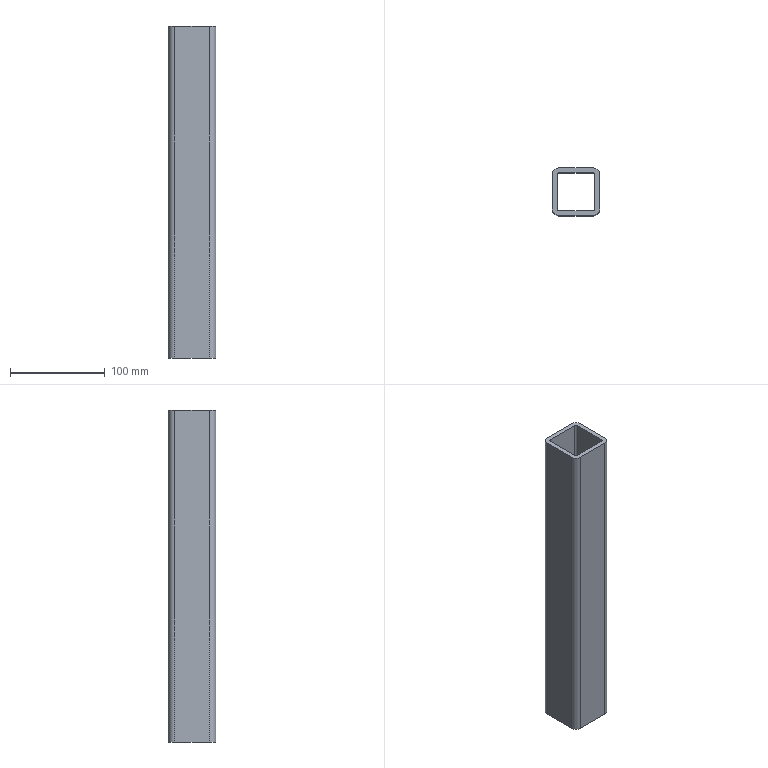Part | NX | 1 solid | 18 faces | box 50 x 50 x 350 mm | volume 301480 mm3 | plane 10 | cylinder 8 | commonest cylinder face diameters 4 x4 14 x4
STEP:
#1=CARTESIAN_POINT('',(-645.,143.,175.));
#2=VERTEX_POINT('',#1);
#3=CARTESIAN_POINT('',(-645.,143.,-175.));
#4=VERTEX_POINT('',#3);
#5=CARTESIAN_POINT('',(-645.,143.,200.));
#6=DIRECTION('',(0.,0.,-1.));
#7=VECTOR('',#6,1000.);
#8=LINE('',#5,#7);
#9=EDGE_CURVE('',#2,#4,#8,.T.);
#10=ORIENTED_EDGE('',*,*,#9,.T.);
#11=CARTESIAN_POINT('',(-645.,179.,-175.));
#12=VERTEX_POINT('',#11);
#13=CARTESIAN_POINT('',(-645.,143.,-175.));
#14=DIRECTION('',(0.,1.,0.));
#15=VECTOR('',#14,1000.);
#16=LINE('',#13,#15);
#17=EDGE_CURVE('',#4,#12,#16,.T.);
#18=ORIENTED_EDGE('',*,*,#17,.T.);
#19=CARTESIAN_POINT('',(-645.,179.,175.));
#20=VERTEX_POINT('',#19);
#21=CARTESIAN_POINT('',(-645.,179.,200.));
#22=DIRECTION('',(0.,0.,-1.));
#23=VECTOR('',#22,1000.);
#24=LINE('',#21,#23);
#25=EDGE_CURVE('',#20,#12,#24,.T.);
#26=ORIENTED_EDGE('',*,*,#25,.F.);
#27=CARTESIAN_POINT('',(-645.,143.,175.));
#28=DIRECTION('',(0.,-1.,0.));
#29=VECTOR('',#28,1000.);
#30=LINE('',#27,#29);
#31=EDGE_CURVE('',#20,#2,#30,.T.);
#32=ORIENTED_EDGE('',*,*,#31,.T.);
#33=EDGE_LOOP('',(#10,#18,#26,#32));
#34=FACE_BOUND('',#33,.T.);
#35=CARTESIAN_POINT('',(-645.,143.,200.));
#36=DIRECTION('',(1.,0.,0.));
#37=DIRECTION('',(0.,0.,-1.));
#38=AXIS2_PLACEMENT_3D('',#35,#36,#37);
#39=PLANE('',#38);
#40=ADVANCED_FACE('',(#34),#39,.T.);
#41=CARTESIAN_POINT('',(-643.,141.,175.));
#42=VERTEX_POINT('',#41);
#43=CARTESIAN_POINT('',(-643.,141.,-175.));
#44=VERTEX_POINT('',#43);
#45=CARTESIAN_POINT('',(-643.,141.,200.));
#46=DIRECTION('',(0.,0.,-1.));
#47=VECTOR('',#46,1000.);
#48=LINE('',#45,#47);
#49=EDGE_CURVE('',#42,#44,#48,.T.);
#50=ORIENTED_EDGE('',*,*,#49,.T.);
#51=CARTESIAN_POINT('',(-643.,143.,-175.));
#52=DIRECTION('',(0.,0.,-1.));
#53=DIRECTION('',(-1.,0.,0.));
#54=AXIS2_PLACEMENT_3D('',#51,#52,#53);
#55=CIRCLE('',#54,2.);
#56=EDGE_CURVE('',#44,#4,#55,.T.);
#57=ORIENTED_EDGE('',*,*,#56,.T.);
#58=ORIENTED_EDGE('',*,*,#9,.F.);
#59=CARTESIAN_POINT('',(-643.,143.,175.));
#60=DIRECTION('',(0.,0.,1.));
#61=DIRECTION('',(1.,0.,0.));
#62=AXIS2_PLACEMENT_3D('',#59,#60,#61);
#63=CIRCLE('',#62,2.);
#64=EDGE_CURVE('',#2,#42,#63,.T.);
#65=ORIENTED_EDGE('',*,*,#64,.T.);
#66=EDGE_LOOP('',(#50,#57,#58,#65));
#67=FACE_BOUND('',#66,.T.);
#68=CARTESIAN_POINT('',(-643.,143.,200.));
#69=DIRECTION('',(0.,0.,-1.));
#70=DIRECTION('',(-1.,0.,0.));
#71=AXIS2_PLACEMENT_3D('',#68,#69,#70);
#72=CYLINDRICAL_SURFACE('',#71,2.);
#73=ADVANCED_FACE('',(#67),#72,.F.);
#74=CARTESIAN_POINT('',(-607.,141.,175.));
#75=VERTEX_POINT('',#74);
#76=CARTESIAN_POINT('',(-607.,141.,-175.));
#77=VERTEX_POINT('',#76);
#78=CARTESIAN_POINT('',(-607.,141.,200.));
#79=DIRECTION('',(0.,0.,-1.));
#80=VECTOR('',#79,1000.);
#81=LINE('',#78,#80);
#82=EDGE_CURVE('',#75,#77,#81,.T.);
#83=ORIENTED_EDGE('',*,*,#82,.T.);
#84=CARTESIAN_POINT('',(-643.,141.,-175.));
#85=DIRECTION('',(-1.,0.,0.));
#86=VECTOR('',#85,1000.);
#87=LINE('',#84,#86);
#88=EDGE_CURVE('',#77,#44,#87,.T.);
#89=ORIENTED_EDGE('',*,*,#88,.T.);
#90=ORIENTED_EDGE('',*,*,#49,.F.);
#91=CARTESIAN_POINT('',(-643.,141.,175.));
#92=DIRECTION('',(1.,0.,0.));
#93=VECTOR('',#92,1000.);
#94=LINE('',#91,#93);
#95=EDGE_CURVE('',#42,#75,#94,.T.);
#96=ORIENTED_EDGE('',*,*,#95,.T.);
#97=EDGE_LOOP('',(#83,#89,#90,#96));
#98=FACE_BOUND('',#97,.T.);
#99=CARTESIAN_POINT('',(-643.,141.,200.));
#100=DIRECTION('',(0.,1.,0.));
#101=DIRECTION('',(-1.,0.,0.));
#102=AXIS2_PLACEMENT_3D('',#99,#100,#101);
#103=PLANE('',#102);
#104=ADVANCED_FACE('',(#98),#103,.T.);
#105=CARTESIAN_POINT('',(-605.,143.,175.));
#106=VERTEX_POINT('',#105);
#107=CARTESIAN_POINT('',(-605.,143.,-175.));
#108=VERTEX_POINT('',#107);
#109=CARTESIAN_POINT('',(-605.,143.,200.));
#110=DIRECTION('',(0.,0.,-1.));
#111=VECTOR('',#110,1000.);
#112=LINE('',#109,#111);
#113=EDGE_CURVE('',#106,#108,#112,.T.);
#114=ORIENTED_EDGE('',*,*,#113,.T.);
#115=CARTESIAN_POINT('',(-607.,143.,-175.));
#116=DIRECTION('',(0.,0.,-1.));
#117=DIRECTION('',(-1.,0.,0.));
#118=AXIS2_PLACEMENT_3D('',#115,#116,#117);
#119=CIRCLE('',#118,2.);
#120=EDGE_CURVE('',#108,#77,#119,.T.);
#121=ORIENTED_EDGE('',*,*,#120,.T.);
#122=ORIENTED_EDGE('',*,*,#82,.F.);
#123=CARTESIAN_POINT('',(-607.,143.,175.));
#124=DIRECTION('',(0.,0.,1.));
#125=DIRECTION('',(1.,0.,0.));
#126=AXIS2_PLACEMENT_3D('',#123,#124,#125);
#127=CIRCLE('',#126,2.);
#128=EDGE_CURVE('',#75,#106,#127,.T.);
#129=ORIENTED_EDGE('',*,*,#128,.T.);
#130=EDGE_LOOP('',(#114,#121,#122,#129));
#131=FACE_BOUND('',#130,.T.);
#132=CARTESIAN_POINT('',(-607.,143.,200.));
#133=DIRECTION('',(0.,0.,-1.));
#134=DIRECTION('',(-1.,0.,0.));
#135=AXIS2_PLACEMENT_3D('',#132,#133,#134);
#136=CYLINDRICAL_SURFACE('',#135,2.);
#137=ADVANCED_FACE('',(#131),#136,.F.);
#138=CARTESIAN_POINT('',(-605.,179.,175.));
#139=VERTEX_POINT('',#138);
#140=CARTESIAN_POINT('',(-605.,179.,-175.));
#141=VERTEX_POINT('',#140);
#142=CARTESIAN_POINT('',(-605.,179.,200.));
#143=DIRECTION('',(0.,0.,-1.));
#144=VECTOR('',#143,1000.);
#145=LINE('',#142,#144);
#146=EDGE_CURVE('',#139,#141,#145,.T.);
#147=ORIENTED_EDGE('',*,*,#146,.T.);
#148=CARTESIAN_POINT('',(-605.,179.,-175.));
#149=DIRECTION('',(0.,-1.,0.));
#150=VECTOR('',#149,1000.);
#151=LINE('',#148,#150);
#152=EDGE_CURVE('',#141,#108,#151,.T.);
#153=ORIENTED_EDGE('',*,*,#152,.T.);
#154=ORIENTED_EDGE('',*,*,#113,.F.);
#155=CARTESIAN_POINT('',(-605.,179.,175.));
#156=DIRECTION('',(0.,1.,0.));
#157=VECTOR('',#156,1000.);
#158=LINE('',#155,#157);
#159=EDGE_CURVE('',#106,#139,#158,.T.);
#160=ORIENTED_EDGE('',*,*,#159,.T.);
#161=EDGE_LOOP('',(#147,#153,#154,#160));
#162=FACE_BOUND('',#161,.T.);
#163=CARTESIAN_POINT('',(-605.,179.,200.));
#164=DIRECTION('',(-1.,0.,0.));
#165=DIRECTION('',(0.,0.,1.));
#166=AXIS2_PLACEMENT_3D('',#163,#164,#165);
#167=PLANE('',#166);
#168=ADVANCED_FACE('',(#162),#167,.T.);
#169=CARTESIAN_POINT('',(-607.,181.,175.));
#170=VERTEX_POINT('',#169);
#171=CARTESIAN_POINT('',(-607.,181.,-175.));
#172=VERTEX_POINT('',#171);
#173=CARTESIAN_POINT('',(-607.,181.,200.));
#174=DIRECTION('',(0.,0.,-1.));
#175=VECTOR('',#174,1000.);
#176=LINE('',#173,#175);
#177=EDGE_CURVE('',#170,#172,#176,.T.);
#178=ORIENTED_EDGE('',*,*,#177,.T.);
#179=CARTESIAN_POINT('',(-607.,179.,-175.));
#180=DIRECTION('',(0.,0.,-1.));
#181=DIRECTION('',(-1.,0.,0.));
#182=AXIS2_PLACEMENT_3D('',#179,#180,#181);
#183=CIRCLE('',#182,2.);
#184=EDGE_CURVE('',#172,#141,#183,.T.);
#185=ORIENTED_EDGE('',*,*,#184,.T.);
#186=ORIENTED_EDGE('',*,*,#146,.F.);
#187=CARTESIAN_POINT('',(-607.,179.,175.));
#188=DIRECTION('',(0.,0.,1.));
#189=DIRECTION('',(1.,0.,0.));
#190=AXIS2_PLACEMENT_3D('',#187,#188,#189);
#191=CIRCLE('',#190,2.);
#192=EDGE_CURVE('',#139,#170,#191,.T.);
#193=ORIENTED_EDGE('',*,*,#192,.T.);
#194=EDGE_LOOP('',(#178,#185,#186,#193));
#195=FACE_BOUND('',#194,.T.);
#196=CARTESIAN_POINT('',(-607.,179.,200.));
#197=DIRECTION('',(0.,0.,-1.));
#198=DIRECTION('',(-1.,0.,0.));
#199=AXIS2_PLACEMENT_3D('',#196,#197,#198);
#200=CYLINDRICAL_SURFACE('',#199,2.);
#201=ADVANCED_FACE('',(#195),#200,.F.);
#202=CARTESIAN_POINT('',(-643.,181.,175.));
#203=VERTEX_POINT('',#202);
#204=CARTESIAN_POINT('',(-643.,181.,-175.));
#205=VERTEX_POINT('',#204);
#206=CARTESIAN_POINT('',(-643.,181.,200.));
#207=DIRECTION('',(0.,0.,-1.));
#208=VECTOR('',#207,1000.);
#209=LINE('',#206,#208);
#210=EDGE_CURVE('',#203,#205,#209,.T.);
#211=ORIENTED_EDGE('',*,*,#210,.T.);
#212=CARTESIAN_POINT('',(-607.,181.,-175.));
#213=DIRECTION('',(1.,0.,0.));
#214=VECTOR('',#213,1000.);
#215=LINE('',#212,#214);
#216=EDGE_CURVE('',#205,#172,#215,.T.);
#217=ORIENTED_EDGE('',*,*,#216,.T.);
#218=ORIENTED_EDGE('',*,*,#177,.F.);
#219=CARTESIAN_POINT('',(-607.,181.,175.));
#220=DIRECTION('',(-1.,0.,0.));
#221=VECTOR('',#220,1000.);
#222=LINE('',#219,#221);
#223=EDGE_CURVE('',#170,#203,#222,.T.);
#224=ORIENTED_EDGE('',*,*,#223,.T.);
#225=EDGE_LOOP('',(#211,#217,#218,#224));
#226=FACE_BOUND('',#225,.T.);
#227=CARTESIAN_POINT('',(-607.,181.,200.));
#228=DIRECTION('',(0.,-1.,0.));
#229=DIRECTION('',(1.,0.,0.));
#230=AXIS2_PLACEMENT_3D('',#227,#228,#229);
#231=PLANE('',#230);
#232=ADVANCED_FACE('',(#226),#231,.T.);
#233=ORIENTED_EDGE('',*,*,#25,.T.);
#234=CARTESIAN_POINT('',(-643.,179.,-175.));
#235=DIRECTION('',(0.,0.,-1.));
#236=DIRECTION('',(-1.,0.,0.));
#237=AXIS2_PLACEMENT_3D('',#234,#235,#236);
#238=CIRCLE('',#237,2.);
#239=EDGE_CURVE('',#12,#205,#238,.T.);
#240=ORIENTED_EDGE('',*,*,#239,.T.);
#241=ORIENTED_EDGE('',*,*,#210,.F.);
#242=CARTESIAN_POINT('',(-643.,179.,175.));
#243=DIRECTION('',(0.,0.,1.));
#244=DIRECTION('',(1.,0.,0.));
#245=AXIS2_PLACEMENT_3D('',#242,#243,#244);
#246=CIRCLE('',#245,2.);
#247=EDGE_CURVE('',#203,#20,#246,.T.);
#248=ORIENTED_EDGE('',*,*,#247,.T.);
#249=EDGE_LOOP('',(#233,#240,#241,#248));
#250=FACE_BOUND('',#249,.T.);
#251=CARTESIAN_POINT('',(-643.,179.,200.));
#252=DIRECTION('',(0.,0.,-1.));
#253=DIRECTION('',(-1.,0.,0.));
#254=AXIS2_PLACEMENT_3D('',#251,#252,#253);
#255=CYLINDRICAL_SURFACE('',#254,2.);
#256=ADVANCED_FACE('',(#250),#255,.F.);
#257=CARTESIAN_POINT('',(-600.,179.,-175.));
#258=VERTEX_POINT('',#257);
#259=CARTESIAN_POINT('',(-600.,143.,-175.));
#260=VERTEX_POINT('',#259);
#261=CARTESIAN_POINT('',(-600.,179.,-175.));
#262=DIRECTION('',(0.,-1.,0.));
#263=VECTOR('',#262,1000.);
#264=LINE('',#261,#263);
#265=EDGE_CURVE('',#258,#260,#264,.T.);
#266=ORIENTED_EDGE('',*,*,#265,.F.);
#267=CARTESIAN_POINT('',(-600.,179.,175.));
#268=VERTEX_POINT('',#267);
#269=CARTESIAN_POINT('',(-600.,179.,200.));
#270=DIRECTION('',(0.,0.,-1.));
#271=VECTOR('',#270,1000.);
#272=LINE('',#269,#271);
#273=EDGE_CURVE('',#268,#258,#272,.T.);
#274=ORIENTED_EDGE('',*,*,#273,.F.);
#275=CARTESIAN_POINT('',(-600.,143.,175.));
#276=VERTEX_POINT('',#275);
#277=CARTESIAN_POINT('',(-600.,179.,175.));
#278=DIRECTION('',(0.,1.,0.));
#279=VECTOR('',#278,1000.);
#280=LINE('',#277,#279);
#281=EDGE_CURVE('',#276,#268,#280,.T.);
#282=ORIENTED_EDGE('',*,*,#281,.F.);
#283=CARTESIAN_POINT('',(-600.,143.,200.));
#284=DIRECTION('',(0.,0.,-1.));
#285=VECTOR('',#284,1000.);
#286=LINE('',#283,#285);
#287=EDGE_CURVE('',#276,#260,#286,.T.);
#288=ORIENTED_EDGE('',*,*,#287,.T.);
#289=EDGE_LOOP('',(#266,#274,#282,#288));
#290=FACE_BOUND('',#289,.T.);
#291=CARTESIAN_POINT('',(-600.,179.,200.));
#292=DIRECTION('',(-1.,0.,0.));
#293=DIRECTION('',(0.,0.,1.));
#294=AXIS2_PLACEMENT_3D('',#291,#292,#293);
#295=PLANE('',#294);
#296=ADVANCED_FACE('',(#290),#295,.F.);
#297=CARTESIAN_POINT('',(-607.,136.,-175.));
#298=VERTEX_POINT('',#297);
#299=CARTESIAN_POINT('',(-607.,143.,-175.));
#300=DIRECTION('',(0.,0.,-1.));
#301=DIRECTION('',(-1.,0.,0.));
#302=AXIS2_PLACEMENT_3D('',#299,#300,#301);
#303=CIRCLE('',#302,7.);
#304=EDGE_CURVE('',#260,#298,#303,.T.);
#305=ORIENTED_EDGE('',*,*,#304,.F.);
#306=ORIENTED_EDGE('',*,*,#287,.F.);
#307=CARTESIAN_POINT('',(-607.,136.,175.));
#308=VERTEX_POINT('',#307);
#309=CARTESIAN_POINT('',(-607.,143.,175.));
#310=DIRECTION('',(0.,0.,1.));
#311=DIRECTION('',(1.,0.,0.));
#312=AXIS2_PLACEMENT_3D('',#309,#310,#311);
#313=CIRCLE('',#312,7.);
#314=EDGE_CURVE('',#308,#276,#313,.T.);
#315=ORIENTED_EDGE('',*,*,#314,.F.);
#316=CARTESIAN_POINT('',(-607.,136.,200.));
#317=DIRECTION('',(0.,0.,-1.));
#318=VECTOR('',#317,1000.);
#319=LINE('',#316,#318);
#320=EDGE_CURVE('',#308,#298,#319,.T.);
#321=ORIENTED_EDGE('',*,*,#320,.T.);
#322=EDGE_LOOP('',(#305,#306,#315,#321));
#323=FACE_BOUND('',#322,.T.);
#324=CARTESIAN_POINT('',(-607.,143.,200.));
#325=DIRECTION('',(0.,0.,-1.));
#326=DIRECTION('',(-1.,0.,0.));
#327=AXIS2_PLACEMENT_3D('',#324,#325,#326);
#328=CYLINDRICAL_SURFACE('',#327,7.);
#329=ADVANCED_FACE('',(#323),#328,.T.);
#330=CARTESIAN_POINT('',(-643.,136.,-175.));
#331=VERTEX_POINT('',#330);
#332=CARTESIAN_POINT('',(-625.,136.,-175.));
#333=DIRECTION('',(1.,0.,0.));
#334=VECTOR('',#333,1000.);
#335=LINE('',#332,#334);
#336=EDGE_CURVE('',#331,#298,#335,.T.);
#337=ORIENTED_EDGE('',*,*,#336,.T.);
#338=ORIENTED_EDGE('',*,*,#320,.F.);
#339=CARTESIAN_POINT('',(-643.,136.,175.));
#340=VERTEX_POINT('',#339);
#341=CARTESIAN_POINT('',(-625.,136.,175.));
#342=DIRECTION('',(1.,0.,0.));
#343=VECTOR('',#342,1000.);
#344=LINE('',#341,#343);
#345=EDGE_CURVE('',#340,#308,#344,.T.);
#346=ORIENTED_EDGE('',*,*,#345,.F.);
#347=CARTESIAN_POINT('',(-643.,136.,200.));
#348=DIRECTION('',(0.,0.,-1.));
#349=VECTOR('',#348,1000.);
#350=LINE('',#347,#349);
#351=EDGE_CURVE('',#340,#331,#350,.T.);
#352=ORIENTED_EDGE('',*,*,#351,.T.);
#353=EDGE_LOOP('',(#337,#338,#346,#352));
#354=FACE_BOUND('',#353,.T.);
#355=CARTESIAN_POINT('',(-643.,136.,200.));
#356=DIRECTION('',(0.,1.,0.));
#357=DIRECTION('',(-1.,0.,0.));
#358=AXIS2_PLACEMENT_3D('',#355,#356,#357);
#359=PLANE('',#358);
#360=ADVANCED_FACE('',(#354),#359,.F.);
#361=CARTESIAN_POINT('',(-650.,143.,-175.));
#362=VERTEX_POINT('',#361);
#363=CARTESIAN_POINT('',(-643.,143.,-175.));
#364=DIRECTION('',(0.,0.,-1.));
#365=DIRECTION('',(-1.,0.,0.));
#366=AXIS2_PLACEMENT_3D('',#363,#364,#365);
#367=CIRCLE('',#366,7.);
#368=EDGE_CURVE('',#331,#362,#367,.T.);
#369=ORIENTED_EDGE('',*,*,#368,.F.);
#370=ORIENTED_EDGE('',*,*,#351,.F.);
#371=CARTESIAN_POINT('',(-650.,143.,175.));
#372=VERTEX_POINT('',#371);
#373=CARTESIAN_POINT('',(-643.,143.,175.));
#374=DIRECTION('',(0.,0.,1.));
#375=DIRECTION('',(1.,0.,0.));
#376=AXIS2_PLACEMENT_3D('',#373,#374,#375);
#377=CIRCLE('',#376,7.);
#378=EDGE_CURVE('',#372,#340,#377,.T.);
#379=ORIENTED_EDGE('',*,*,#378,.F.);
#380=CARTESIAN_POINT('',(-650.,143.,200.));
#381=DIRECTION('',(0.,0.,-1.));
#382=VECTOR('',#381,1000.);
#383=LINE('',#380,#382);
#384=EDGE_CURVE('',#372,#362,#383,.T.);
#385=ORIENTED_EDGE('',*,*,#384,.T.);
#386=EDGE_LOOP('',(#369,#370,#379,#385));
#387=FACE_BOUND('',#386,.T.);
#388=CARTESIAN_POINT('',(-643.,143.,200.));
#389=DIRECTION('',(0.,0.,-1.));
#390=DIRECTION('',(-1.,0.,0.));
#391=AXIS2_PLACEMENT_3D('',#388,#389,#390);
#392=CYLINDRICAL_SURFACE('',#391,7.);
#393=ADVANCED_FACE('',(#387),#392,.T.);
#394=CARTESIAN_POINT('',(-650.,179.,-175.));
#395=VERTEX_POINT('',#394);
#396=CARTESIAN_POINT('',(-650.,143.,-175.));
#397=DIRECTION('',(0.,1.,0.));
#398=VECTOR('',#397,1000.);
#399=LINE('',#396,#398);
#400=EDGE_CURVE('',#362,#395,#399,.T.);
#401=ORIENTED_EDGE('',*,*,#400,.F.);
#402=ORIENTED_EDGE('',*,*,#384,.F.);
#403=CARTESIAN_POINT('',(-650.,179.,175.));
#404=VERTEX_POINT('',#403);
#405=CARTESIAN_POINT('',(-650.,143.,175.));
#406=DIRECTION('',(0.,-1.,0.));
#407=VECTOR('',#406,1000.);
#408=LINE('',#405,#407);
#409=EDGE_CURVE('',#404,#372,#408,.T.);
#410=ORIENTED_EDGE('',*,*,#409,.F.);
#411=CARTESIAN_POINT('',(-650.,179.,200.));
#412=DIRECTION('',(0.,0.,-1.));
#413=VECTOR('',#412,1000.);
#414=LINE('',#411,#413);
#415=EDGE_CURVE('',#404,#395,#414,.T.);
#416=ORIENTED_EDGE('',*,*,#415,.T.);
#417=EDGE_LOOP('',(#401,#402,#410,#416));
#418=FACE_BOUND('',#417,.T.);
#419=CARTESIAN_POINT('',(-650.,143.,200.));
#420=DIRECTION('',(1.,0.,0.));
#421=DIRECTION('',(0.,0.,-1.));
#422=AXIS2_PLACEMENT_3D('',#419,#420,#421);
#423=PLANE('',#422);
#424=ADVANCED_FACE('',(#418),#423,.F.);
#425=CARTESIAN_POINT('',(-643.,186.,-175.));
#426=VERTEX_POINT('',#425);
#427=CARTESIAN_POINT('',(-643.,179.,-175.));
#428=DIRECTION('',(0.,0.,-1.));
#429=DIRECTION('',(-1.,0.,0.));
#430=AXIS2_PLACEMENT_3D('',#427,#428,#429);
#431=CIRCLE('',#430,7.);
#432=EDGE_CURVE('',#395,#426,#431,.T.);
#433=ORIENTED_EDGE('',*,*,#432,.F.);
#434=ORIENTED_EDGE('',*,*,#415,.F.);
#435=CARTESIAN_POINT('',(-643.,186.,175.));
#436=VERTEX_POINT('',#435);
#437=CARTESIAN_POINT('',(-643.,179.,175.));
#438=DIRECTION('',(0.,0.,1.));
#439=DIRECTION('',(1.,0.,0.));
#440=AXIS2_PLACEMENT_3D('',#437,#438,#439);
#441=CIRCLE('',#440,7.);
#442=EDGE_CURVE('',#436,#404,#441,.T.);
#443=ORIENTED_EDGE('',*,*,#442,.F.);
#444=CARTESIAN_POINT('',(-643.,186.,200.));
#445=DIRECTION('',(0.,0.,-1.));
#446=VECTOR('',#445,1000.);
#447=LINE('',#444,#446);
#448=EDGE_CURVE('',#436,#426,#447,.T.);
#449=ORIENTED_EDGE('',*,*,#448,.T.);
#450=EDGE_LOOP('',(#433,#434,#443,#449));
#451=FACE_BOUND('',#450,.T.);
#452=CARTESIAN_POINT('',(-643.,179.,200.));
#453=DIRECTION('',(0.,0.,-1.));
#454=DIRECTION('',(-1.,0.,0.));
#455=AXIS2_PLACEMENT_3D('',#452,#453,#454);
#456=CYLINDRICAL_SURFACE('',#455,7.);
#457=ADVANCED_FACE('',(#451),#456,.T.);
#458=CARTESIAN_POINT('',(-607.,186.,-175.));
#459=VERTEX_POINT('',#458);
#460=CARTESIAN_POINT('',(-625.,186.,-175.));
#461=DIRECTION('',(1.,0.,0.));
#462=VECTOR('',#461,1000.);
#463=LINE('',#460,#462);
#464=EDGE_CURVE('',#426,#459,#463,.T.);
#465=ORIENTED_EDGE('',*,*,#464,.F.);
#466=ORIENTED_EDGE('',*,*,#448,.F.);
#467=CARTESIAN_POINT('',(-607.,186.,175.));
#468=VERTEX_POINT('',#467);
#469=CARTESIAN_POINT('',(-625.,186.,175.));
#470=DIRECTION('',(1.,0.,0.));
#471=VECTOR('',#470,1000.);
#472=LINE('',#469,#471);
#473=EDGE_CURVE('',#436,#468,#472,.T.);
#474=ORIENTED_EDGE('',*,*,#473,.T.);
#475=CARTESIAN_POINT('',(-607.,186.,200.));
#476=DIRECTION('',(0.,0.,-1.));
#477=VECTOR('',#476,1000.);
#478=LINE('',#475,#477);
#479=EDGE_CURVE('',#468,#459,#478,.T.);
#480=ORIENTED_EDGE('',*,*,#479,.T.);
#481=EDGE_LOOP('',(#465,#466,#474,#480));
#482=FACE_BOUND('',#481,.T.);
#483=CARTESIAN_POINT('',(-607.,186.,200.));
#484=DIRECTION('',(0.,-1.,0.));
#485=DIRECTION('',(1.,0.,0.));
#486=AXIS2_PLACEMENT_3D('',#483,#484,#485);
#487=PLANE('',#486);
#488=ADVANCED_FACE('',(#482),#487,.F.);
#489=CARTESIAN_POINT('',(-607.,179.,-175.));
#490=DIRECTION('',(0.,0.,-1.));
#491=DIRECTION('',(-1.,0.,0.));
#492=AXIS2_PLACEMENT_3D('',#489,#490,#491);
#493=CIRCLE('',#492,7.);
#494=EDGE_CURVE('',#459,#258,#493,.T.);
#495=ORIENTED_EDGE('',*,*,#494,.F.);
#496=ORIENTED_EDGE('',*,*,#479,.F.);
#497=CARTESIAN_POINT('',(-607.,179.,175.));
#498=DIRECTION('',(0.,0.,1.));
#499=DIRECTION('',(1.,0.,0.));
#500=AXIS2_PLACEMENT_3D('',#497,#498,#499);
#501=CIRCLE('',#500,7.);
#502=EDGE_CURVE('',#268,#468,#501,.T.);
#503=ORIENTED_EDGE('',*,*,#502,.F.);
#504=ORIENTED_EDGE('',*,*,#273,.T.);
#505=EDGE_LOOP('',(#495,#496,#503,#504));
#506=FACE_BOUND('',#505,.T.);
#507=CARTESIAN_POINT('',(-607.,179.,200.));
#508=DIRECTION('',(0.,0.,-1.));
#509=DIRECTION('',(-1.,0.,0.));
#510=AXIS2_PLACEMENT_3D('',#507,#508,#509);
#511=CYLINDRICAL_SURFACE('',#510,7.);
#512=ADVANCED_FACE('',(#506),#511,.T.);
#513=ORIENTED_EDGE('',*,*,#223,.F.);
#514=ORIENTED_EDGE('',*,*,#192,.F.);
#515=ORIENTED_EDGE('',*,*,#159,.F.);
#516=ORIENTED_EDGE('',*,*,#128,.F.);
#517=ORIENTED_EDGE('',*,*,#95,.F.);
#518=ORIENTED_EDGE('',*,*,#64,.F.);
#519=ORIENTED_EDGE('',*,*,#31,.F.);
#520=ORIENTED_EDGE('',*,*,#247,.F.);
#521=EDGE_LOOP('',(#513,#514,#515,#516,#517,#518,#519,#520));
#522=FACE_BOUND('',#521,.T.);
#523=ORIENTED_EDGE('',*,*,#442,.T.);
#524=ORIENTED_EDGE('',*,*,#409,.T.);
#525=ORIENTED_EDGE('',*,*,#378,.T.);
#526=ORIENTED_EDGE('',*,*,#345,.T.);
#527=ORIENTED_EDGE('',*,*,#314,.T.);
#528=ORIENTED_EDGE('',*,*,#281,.T.);
#529=ORIENTED_EDGE('',*,*,#502,.T.);
#530=ORIENTED_EDGE('',*,*,#473,.F.);
#531=EDGE_LOOP('',(#523,#524,#525,#526,#527,#528,#529,#530));
#532=FACE_BOUND('',#531,.T.);
#533=CARTESIAN_POINT('',(-625.,143.,175.));
#534=DIRECTION('',(0.,0.,1.));
#535=DIRECTION('',(1.,0.,0.));
#536=AXIS2_PLACEMENT_3D('',#533,#534,#535);
#537=PLANE('',#536);
#538=ADVANCED_FACE('',(#522,#532),#537,.T.);
#539=ORIENTED_EDGE('',*,*,#56,.F.);
#540=ORIENTED_EDGE('',*,*,#88,.F.);
#541=ORIENTED_EDGE('',*,*,#120,.F.);
#542=ORIENTED_EDGE('',*,*,#152,.F.);
#543=ORIENTED_EDGE('',*,*,#184,.F.);
#544=ORIENTED_EDGE('',*,*,#216,.F.);
#545=ORIENTED_EDGE('',*,*,#239,.F.);
#546=ORIENTED_EDGE('',*,*,#17,.F.);
#547=EDGE_LOOP('',(#539,#540,#541,#542,#543,#544,#545,#546));
#548=FACE_BOUND('',#547,.T.);
#549=ORIENTED_EDGE('',*,*,#368,.T.);
#550=ORIENTED_EDGE('',*,*,#400,.T.);
#551=ORIENTED_EDGE('',*,*,#432,.T.);
#552=ORIENTED_EDGE('',*,*,#464,.T.);
#553=ORIENTED_EDGE('',*,*,#494,.T.);
#554=ORIENTED_EDGE('',*,*,#265,.T.);
#555=ORIENTED_EDGE('',*,*,#304,.T.);
#556=ORIENTED_EDGE('',*,*,#336,.F.);
#557=EDGE_LOOP('',(#549,#550,#551,#552,#553,#554,#555,#556));
#558=FACE_BOUND('',#557,.T.);
#559=CARTESIAN_POINT('',(-625.,179.,-175.));
#560=DIRECTION('',(0.,0.,-1.));
#561=DIRECTION('',(-1.,0.,0.));
#562=AXIS2_PLACEMENT_3D('',#559,#560,#561);
#563=PLANE('',#562);
#564=ADVANCED_FACE('',(#548,#558),#563,.T.);
#565=CLOSED_SHELL('',(#40,#73,#104,#137,#168,#201,#232,#256,#296,#329,#360,#393,#424,#457,#488,#512,#538,#564));
#566=MANIFOLD_SOLID_BREP('',#565);
#567=(LENGTH_UNIT()NAMED_UNIT(*)SI_UNIT(.MILLI.,.METRE.));
#568=UNCERTAINTY_MEASURE_WITH_UNIT(LENGTH_MEASURE(0.00001),#567,'','');
#569=(NAMED_UNIT(*)PLANE_ANGLE_UNIT()SI_UNIT($,.RADIAN.));
#570=(NAMED_UNIT(*)SI_UNIT($,.STERADIAN.)SOLID_ANGLE_UNIT());
#571=(GEOMETRIC_REPRESENTATION_CONTEXT(3)GLOBAL_UNCERTAINTY_ASSIGNED_CONTEXT((#568))GLOBAL_UNIT_ASSIGNED_CONTEXT((#567,#569,#570))REPRESENTATION_CONTEXT('',''));
#572=ADVANCED_BREP_SHAPE_REPRESENTATION('',(#566),#571);